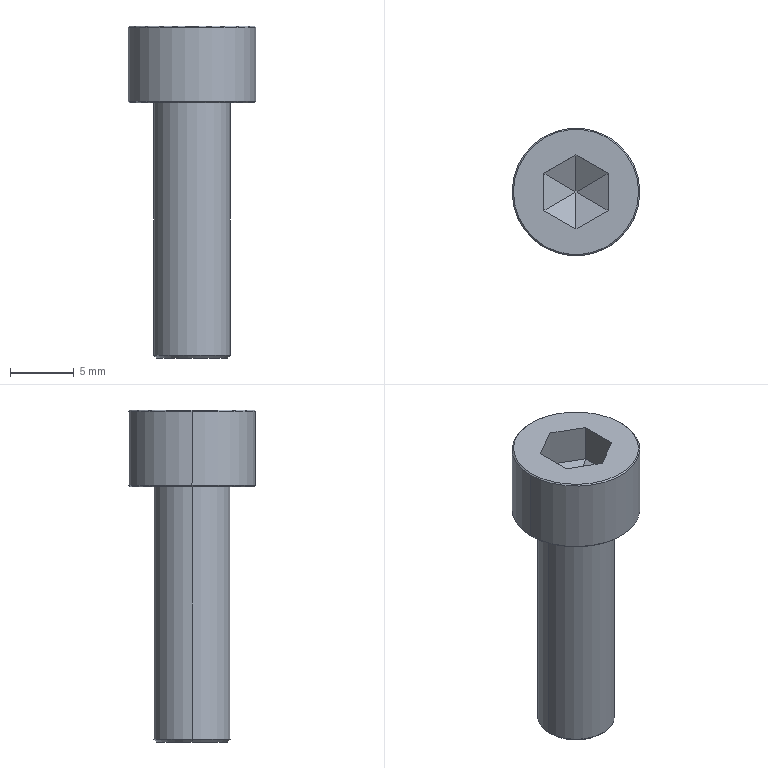Part | SolidWorks | features BaseBody 1 | 1 solid | 26 faces | box 10 x 10 x 26 mm | volume 959.271 mm3 | plane 16 | cone 6 | cylinder 4 | commonest cylinder face diameters 6 x2 10 x2
STEP:
#1=CARTESIAN_POINT('',(3.,0.,0.2));
#2=VERTEX_POINT('',#1);
#3=CARTESIAN_POINT('',(-3.,0.,0.2));
#4=VERTEX_POINT('',#3);
#5=CARTESIAN_POINT('',(0.,0.,0.2));
#6=DIRECTION('',(0.,0.,1.));
#7=DIRECTION('',(1.,0.,0.));
#8=AXIS2_PLACEMENT_3D('',#5,#6,#7);
#9=CIRCLE('',#8,3.);
#10=EDGE_CURVE('',#2,#4,#9,.T.);
#11=ORIENTED_EDGE('',*,*,#10,.T.);
#12=CARTESIAN_POINT('',(-3.,0.,20.));
#13=VERTEX_POINT('',#12);
#14=CARTESIAN_POINT('',(-3.,0.,0.));
#15=DIRECTION('',(0.,0.,1.));
#16=VECTOR('',#15,1000.);
#17=LINE('',#14,#16);
#18=EDGE_CURVE('',#4,#13,#17,.T.);
#19=ORIENTED_EDGE('',*,*,#18,.T.);
#20=CARTESIAN_POINT('',(3.,0.,20.));
#21=VERTEX_POINT('',#20);
#22=CARTESIAN_POINT('',(0.,0.,20.));
#23=DIRECTION('',(0.,0.,-1.));
#24=DIRECTION('',(1.,0.,0.));
#25=AXIS2_PLACEMENT_3D('',#22,#23,#24);
#26=CIRCLE('',#25,3.);
#27=EDGE_CURVE('',#13,#21,#26,.T.);
#28=ORIENTED_EDGE('',*,*,#27,.T.);
#29=CARTESIAN_POINT('',(3.,0.,0.));
#30=DIRECTION('',(0.,0.,1.));
#31=VECTOR('',#30,1000.);
#32=LINE('',#29,#31);
#33=EDGE_CURVE('',#2,#21,#32,.T.);
#34=ORIENTED_EDGE('',*,*,#33,.F.);
#35=EDGE_LOOP('',(#11,#19,#28,#34));
#36=FACE_OUTER_BOUND('',#35,.T.);
#37=CARTESIAN_POINT('',(0.,0.,0.));
#38=DIRECTION('',(0.,0.,1.));
#39=DIRECTION('',(1.,0.,0.));
#40=AXIS2_PLACEMENT_3D('',#37,#38,#39);
#41=CYLINDRICAL_SURFACE('',#40,3.);
#42=ADVANCED_FACE('',(#36),#41,.T.);
#43=CARTESIAN_POINT('',(2.8,0.,0.));
#44=VERTEX_POINT('',#43);
#45=CARTESIAN_POINT('',(-2.8,0.,0.));
#46=VERTEX_POINT('',#45);
#47=CARTESIAN_POINT('',(0.,0.,0.));
#48=DIRECTION('',(0.,0.,1.));
#49=DIRECTION('',(1.,0.,0.));
#50=AXIS2_PLACEMENT_3D('',#47,#48,#49);
#51=CIRCLE('',#50,2.8);
#52=EDGE_CURVE('',#44,#46,#51,.T.);
#53=ORIENTED_EDGE('',*,*,#52,.T.);
#54=CARTESIAN_POINT('',(-3.,0.,0.2));
#55=DIRECTION('',(-0.7071,0.,0.7071));
#56=VECTOR('',#55,1000.);
#57=LINE('',#54,#56);
#58=EDGE_CURVE('',#46,#4,#57,.T.);
#59=ORIENTED_EDGE('',*,*,#58,.T.);
#60=ORIENTED_EDGE('',*,*,#10,.F.);
#61=CARTESIAN_POINT('',(3.,0.,0.2));
#62=DIRECTION('',(0.7071,0.,0.7071));
#63=VECTOR('',#62,1000.);
#64=LINE('',#61,#63);
#65=EDGE_CURVE('',#44,#2,#64,.T.);
#66=ORIENTED_EDGE('',*,*,#65,.F.);
#67=EDGE_LOOP('',(#53,#59,#60,#66));
#68=FACE_OUTER_BOUND('',#67,.T.);
#69=CARTESIAN_POINT('',(0.,0.,0.2));
#70=DIRECTION('',(0.,0.,1.));
#71=DIRECTION('',(1.,0.,0.));
#72=AXIS2_PLACEMENT_3D('',#69,#70,#71);
#73=CONICAL_SURFACE('',#72,3.,0.7854);
#74=ADVANCED_FACE('',(#68),#73,.T.);
#75=CARTESIAN_POINT('',(4.9,0.,20.));
#76=VERTEX_POINT('',#75);
#77=CARTESIAN_POINT('',(-4.9,0.,20.));
#78=VERTEX_POINT('',#77);
#79=CARTESIAN_POINT('',(0.,0.,20.));
#80=DIRECTION('',(0.,0.,1.));
#81=DIRECTION('',(1.,0.,0.));
#82=AXIS2_PLACEMENT_3D('',#79,#80,#81);
#83=CIRCLE('',#82,4.9);
#84=EDGE_CURVE('',#76,#78,#83,.T.);
#85=ORIENTED_EDGE('',*,*,#84,.T.);
#86=CARTESIAN_POINT('',(-5.,0.,20.1));
#87=VERTEX_POINT('',#86);
#88=CARTESIAN_POINT('',(-5.,0.,20.1));
#89=DIRECTION('',(-0.7071,0.,0.7071));
#90=VECTOR('',#89,1000.);
#91=LINE('',#88,#90);
#92=EDGE_CURVE('',#78,#87,#91,.T.);
#93=ORIENTED_EDGE('',*,*,#92,.T.);
#94=CARTESIAN_POINT('',(5.,0.,20.1));
#95=VERTEX_POINT('',#94);
#96=CARTESIAN_POINT('',(0.,0.,20.1));
#97=DIRECTION('',(0.,0.,-1.));
#98=DIRECTION('',(0.,-1.,0.));
#99=AXIS2_PLACEMENT_3D('',#96,#97,#98);
#100=CIRCLE('',#99,5.);
#101=EDGE_CURVE('',#87,#95,#100,.T.);
#102=ORIENTED_EDGE('',*,*,#101,.T.);
#103=CARTESIAN_POINT('',(5.,0.,20.1));
#104=DIRECTION('',(0.7071,0.,0.7071));
#105=VECTOR('',#104,1000.);
#106=LINE('',#103,#105);
#107=EDGE_CURVE('',#76,#95,#106,.T.);
#108=ORIENTED_EDGE('',*,*,#107,.F.);
#109=EDGE_LOOP('',(#85,#93,#102,#108));
#110=FACE_OUTER_BOUND('',#109,.T.);
#111=CARTESIAN_POINT('',(0.,0.,20.1));
#112=DIRECTION('',(0.,0.,1.));
#113=DIRECTION('',(1.,0.,0.));
#114=AXIS2_PLACEMENT_3D('',#111,#112,#113);
#115=CONICAL_SURFACE('',#114,5.,0.7854);
#116=ADVANCED_FACE('',(#110),#115,.T.);
#117=ORIENTED_EDGE('',*,*,#101,.F.);
#118=CARTESIAN_POINT('',(-5.,0.,25.9));
#119=VERTEX_POINT('',#118);
#120=CARTESIAN_POINT('',(-5.,0.,20.));
#121=DIRECTION('',(0.,0.,1.));
#122=VECTOR('',#121,1000.);
#123=LINE('',#120,#122);
#124=EDGE_CURVE('',#87,#119,#123,.T.);
#125=ORIENTED_EDGE('',*,*,#124,.T.);
#126=CARTESIAN_POINT('',(5.,0.,25.9));
#127=VERTEX_POINT('',#126);
#128=CARTESIAN_POINT('',(0.,0.,25.9));
#129=DIRECTION('',(0.,0.,-1.));
#130=DIRECTION('',(1.,0.,0.));
#131=AXIS2_PLACEMENT_3D('',#128,#129,#130);
#132=CIRCLE('',#131,5.);
#133=EDGE_CURVE('',#119,#127,#132,.T.);
#134=ORIENTED_EDGE('',*,*,#133,.T.);
#135=CARTESIAN_POINT('',(5.,0.,20.));
#136=DIRECTION('',(0.,0.,1.));
#137=VECTOR('',#136,1000.);
#138=LINE('',#135,#137);
#139=EDGE_CURVE('',#95,#127,#138,.T.);
#140=ORIENTED_EDGE('',*,*,#139,.F.);
#141=EDGE_LOOP('',(#117,#125,#134,#140));
#142=FACE_OUTER_BOUND('',#141,.T.);
#143=CARTESIAN_POINT('',(0.,0.,20.));
#144=DIRECTION('',(0.,0.,1.));
#145=DIRECTION('',(1.,0.,0.));
#146=AXIS2_PLACEMENT_3D('',#143,#144,#145);
#147=CYLINDRICAL_SURFACE('',#146,5.);
#148=ADVANCED_FACE('',(#142),#147,.T.);
#149=CARTESIAN_POINT('',(-4.9,0.,26.));
#150=VERTEX_POINT('',#149);
#151=CARTESIAN_POINT('',(4.9,0.,26.));
#152=VERTEX_POINT('',#151);
#153=CARTESIAN_POINT('',(0.,0.,26.));
#154=DIRECTION('',(0.,0.,-1.));
#155=DIRECTION('',(1.,0.,0.));
#156=AXIS2_PLACEMENT_3D('',#153,#154,#155);
#157=CIRCLE('',#156,4.9);
#158=EDGE_CURVE('',#150,#152,#157,.T.);
#159=ORIENTED_EDGE('',*,*,#158,.T.);
#160=CARTESIAN_POINT('',(5.,0.,25.9));
#161=DIRECTION('',(0.7071,0.,-0.7071));
#162=VECTOR('',#161,1000.);
#163=LINE('',#160,#162);
#164=EDGE_CURVE('',#152,#127,#163,.T.);
#165=ORIENTED_EDGE('',*,*,#164,.T.);
#166=ORIENTED_EDGE('',*,*,#133,.F.);
#167=CARTESIAN_POINT('',(-5.,0.,25.9));
#168=DIRECTION('',(-0.7071,0.,-0.7071));
#169=VECTOR('',#168,1000.);
#170=LINE('',#167,#169);
#171=EDGE_CURVE('',#150,#119,#170,.T.);
#172=ORIENTED_EDGE('',*,*,#171,.F.);
#173=EDGE_LOOP('',(#159,#165,#166,#172));
#174=FACE_OUTER_BOUND('',#173,.T.);
#175=CARTESIAN_POINT('',(0.,0.,25.9));
#176=DIRECTION('',(0.,0.,-1.));
#177=DIRECTION('',(-1.,0.,0.));
#178=AXIS2_PLACEMENT_3D('',#175,#176,#177);
#179=CONICAL_SURFACE('',#178,5.,0.7854);
#180=ADVANCED_FACE('',(#174),#179,.T.);
#181=ORIENTED_EDGE('',*,*,#18,.F.);
#182=CARTESIAN_POINT('',(0.,0.,0.2));
#183=DIRECTION('',(0.,0.,1.));
#184=DIRECTION('',(1.,0.,0.));
#185=AXIS2_PLACEMENT_3D('',#182,#183,#184);
#186=CIRCLE('',#185,3.);
#187=EDGE_CURVE('',#4,#2,#186,.T.);
#188=ORIENTED_EDGE('',*,*,#187,.T.);
#189=ORIENTED_EDGE('',*,*,#33,.T.);
#190=CARTESIAN_POINT('',(0.,0.,20.));
#191=DIRECTION('',(0.,0.,-1.));
#192=DIRECTION('',(1.,0.,0.));
#193=AXIS2_PLACEMENT_3D('',#190,#191,#192);
#194=CIRCLE('',#193,3.);
#195=EDGE_CURVE('',#21,#13,#194,.T.);
#196=ORIENTED_EDGE('',*,*,#195,.T.);
#197=EDGE_LOOP('',(#181,#188,#189,#196));
#198=FACE_OUTER_BOUND('',#197,.T.);
#199=CARTESIAN_POINT('',(0.,0.,0.));
#200=DIRECTION('',(0.,0.,1.));
#201=DIRECTION('',(1.,0.,0.));
#202=AXIS2_PLACEMENT_3D('',#199,#200,#201);
#203=CYLINDRICAL_SURFACE('',#202,3.);
#204=ADVANCED_FACE('',(#198),#203,.T.);
#205=ORIENTED_EDGE('',*,*,#58,.F.);
#206=CARTESIAN_POINT('',(0.,0.,0.));
#207=DIRECTION('',(0.,0.,1.));
#208=DIRECTION('',(1.,0.,0.));
#209=AXIS2_PLACEMENT_3D('',#206,#207,#208);
#210=CIRCLE('',#209,2.8);
#211=EDGE_CURVE('',#46,#44,#210,.T.);
#212=ORIENTED_EDGE('',*,*,#211,.T.);
#213=ORIENTED_EDGE('',*,*,#65,.T.);
#214=ORIENTED_EDGE('',*,*,#187,.F.);
#215=EDGE_LOOP('',(#205,#212,#213,#214));
#216=FACE_OUTER_BOUND('',#215,.T.);
#217=CARTESIAN_POINT('',(0.,0.,0.2));
#218=DIRECTION('',(0.,0.,1.));
#219=DIRECTION('',(1.,0.,0.));
#220=AXIS2_PLACEMENT_3D('',#217,#218,#219);
#221=CONICAL_SURFACE('',#220,3.,0.7854);
#222=ADVANCED_FACE('',(#216),#221,.T.);
#223=ORIENTED_EDGE('',*,*,#195,.F.);
#224=ORIENTED_EDGE('',*,*,#27,.F.);
#225=EDGE_LOOP('',(#223,#224));
#226=FACE_BOUND('',#225,.T.);
#227=ORIENTED_EDGE('',*,*,#84,.F.);
#228=CARTESIAN_POINT('',(0.,0.,20.));
#229=DIRECTION('',(0.,0.,1.));
#230=DIRECTION('',(1.,0.,0.));
#231=AXIS2_PLACEMENT_3D('',#228,#229,#230);
#232=CIRCLE('',#231,4.9);
#233=EDGE_CURVE('',#78,#76,#232,.T.);
#234=ORIENTED_EDGE('',*,*,#233,.F.);
#235=EDGE_LOOP('',(#227,#234));
#236=FACE_OUTER_BOUND('',#235,.T.);
#237=CARTESIAN_POINT('',(0.,0.,20.));
#238=DIRECTION('',(0.,0.,1.));
#239=DIRECTION('',(1.,0.,0.));
#240=AXIS2_PLACEMENT_3D('',#237,#238,#239);
#241=PLANE('',#240);
#242=ADVANCED_FACE('',(#226,#236),#241,.F.);
#243=ORIENTED_EDGE('',*,*,#52,.F.);
#244=ORIENTED_EDGE('',*,*,#211,.F.);
#245=EDGE_LOOP('',(#243,#244));
#246=FACE_OUTER_BOUND('',#245,.T.);
#247=CARTESIAN_POINT('',(0.,0.,0.));
#248=DIRECTION('',(0.,0.,1.));
#249=DIRECTION('',(1.,0.,0.));
#250=AXIS2_PLACEMENT_3D('',#247,#248,#249);
#251=PLANE('',#250);
#252=ADVANCED_FACE('',(#246),#251,.F.);
#253=ORIENTED_EDGE('',*,*,#92,.F.);
#254=ORIENTED_EDGE('',*,*,#233,.T.);
#255=ORIENTED_EDGE('',*,*,#107,.T.);
#256=CARTESIAN_POINT('',(0.,0.,20.1));
#257=DIRECTION('',(0.,0.,-1.));
#258=DIRECTION('',(0.,-1.,0.));
#259=AXIS2_PLACEMENT_3D('',#256,#257,#258);
#260=CIRCLE('',#259,5.);
#261=EDGE_CURVE('',#95,#87,#260,.T.);
#262=ORIENTED_EDGE('',*,*,#261,.T.);
#263=EDGE_LOOP('',(#253,#254,#255,#262));
#264=FACE_OUTER_BOUND('',#263,.T.);
#265=CARTESIAN_POINT('',(0.,0.,20.1));
#266=DIRECTION('',(0.,0.,1.));
#267=DIRECTION('',(1.,0.,0.));
#268=AXIS2_PLACEMENT_3D('',#265,#266,#267);
#269=CONICAL_SURFACE('',#268,5.,0.7854);
#270=ADVANCED_FACE('',(#264),#269,.T.);
#271=ORIENTED_EDGE('',*,*,#124,.F.);
#272=ORIENTED_EDGE('',*,*,#261,.F.);
#273=ORIENTED_EDGE('',*,*,#139,.T.);
#274=CARTESIAN_POINT('',(0.,0.,25.9));
#275=DIRECTION('',(0.,0.,-1.));
#276=DIRECTION('',(1.,0.,0.));
#277=AXIS2_PLACEMENT_3D('',#274,#275,#276);
#278=CIRCLE('',#277,5.);
#279=EDGE_CURVE('',#127,#119,#278,.T.);
#280=ORIENTED_EDGE('',*,*,#279,.T.);
#281=EDGE_LOOP('',(#271,#272,#273,#280));
#282=FACE_OUTER_BOUND('',#281,.T.);
#283=CARTESIAN_POINT('',(0.,0.,20.));
#284=DIRECTION('',(0.,0.,1.));
#285=DIRECTION('',(1.,0.,0.));
#286=AXIS2_PLACEMENT_3D('',#283,#284,#285);
#287=CYLINDRICAL_SURFACE('',#286,5.);
#288=ADVANCED_FACE('',(#282),#287,.T.);
#289=ORIENTED_EDGE('',*,*,#164,.F.);
#290=CARTESIAN_POINT('',(0.,0.,26.));
#291=DIRECTION('',(0.,0.,-1.));
#292=DIRECTION('',(1.,0.,0.));
#293=AXIS2_PLACEMENT_3D('',#290,#291,#292);
#294=CIRCLE('',#293,4.9);
#295=EDGE_CURVE('',#152,#150,#294,.T.);
#296=ORIENTED_EDGE('',*,*,#295,.T.);
#297=ORIENTED_EDGE('',*,*,#171,.T.);
#298=ORIENTED_EDGE('',*,*,#279,.F.);
#299=EDGE_LOOP('',(#289,#296,#297,#298));
#300=FACE_OUTER_BOUND('',#299,.T.);
#301=CARTESIAN_POINT('',(0.,0.,25.9));
#302=DIRECTION('',(0.,0.,-1.));
#303=DIRECTION('',(-1.,0.,0.));
#304=AXIS2_PLACEMENT_3D('',#301,#302,#303);
#305=CONICAL_SURFACE('',#304,5.,0.7854);
#306=ADVANCED_FACE('',(#300),#305,.T.);
#307=CARTESIAN_POINT('',(-2.51,-1.449,26.));
#308=VERTEX_POINT('',#307);
#309=CARTESIAN_POINT('',(-2.51,1.449,26.));
#310=VERTEX_POINT('',#309);
#311=CARTESIAN_POINT('',(-2.51,0.,26.));
#312=DIRECTION('',(0.,1.,0.));
#313=VECTOR('',#312,1000.);
#314=LINE('',#311,#313);
#315=EDGE_CURVE('',#308,#310,#314,.T.);
#316=ORIENTED_EDGE('',*,*,#315,.T.);
#317=CARTESIAN_POINT('',(0.,2.898,26.));
#318=VERTEX_POINT('',#317);
#319=CARTESIAN_POINT('',(-2.51,1.449,26.));
#320=DIRECTION('',(0.866,0.5,0.));
#321=VECTOR('',#320,1000.);
#322=LINE('',#319,#321);
#323=EDGE_CURVE('',#310,#318,#322,.T.);
#324=ORIENTED_EDGE('',*,*,#323,.T.);
#325=CARTESIAN_POINT('',(2.51,1.449,26.));
#326=VERTEX_POINT('',#325);
#327=CARTESIAN_POINT('',(0.,2.898,26.));
#328=DIRECTION('',(0.866,-0.5,0.));
#329=VECTOR('',#328,1000.);
#330=LINE('',#327,#329);
#331=EDGE_CURVE('',#318,#326,#330,.T.);
#332=ORIENTED_EDGE('',*,*,#331,.T.);
#333=CARTESIAN_POINT('',(2.51,-1.449,26.));
#334=VERTEX_POINT('',#333);
#335=CARTESIAN_POINT('',(2.51,0.,26.));
#336=DIRECTION('',(0.,-1.,0.));
#337=VECTOR('',#336,1000.);
#338=LINE('',#335,#337);
#339=EDGE_CURVE('',#326,#334,#338,.T.);
#340=ORIENTED_EDGE('',*,*,#339,.T.);
#341=CARTESIAN_POINT('',(0.,-2.898,26.));
#342=VERTEX_POINT('',#341);
#343=CARTESIAN_POINT('',(2.51,-1.449,26.));
#344=DIRECTION('',(-0.866,-0.5,0.));
#345=VECTOR('',#344,1000.);
#346=LINE('',#343,#345);
#347=EDGE_CURVE('',#334,#342,#346,.T.);
#348=ORIENTED_EDGE('',*,*,#347,.T.);
#349=CARTESIAN_POINT('',(0.,-2.898,26.));
#350=DIRECTION('',(-0.866,0.5,0.));
#351=VECTOR('',#350,1000.);
#352=LINE('',#349,#351);
#353=EDGE_CURVE('',#342,#308,#352,.T.);
#354=ORIENTED_EDGE('',*,*,#353,.T.);
#355=EDGE_LOOP('',(#316,#324,#332,#340,#348,#354));
#356=FACE_BOUND('',#355,.T.);
#357=ORIENTED_EDGE('',*,*,#158,.F.);
#358=ORIENTED_EDGE('',*,*,#295,.F.);
#359=EDGE_LOOP('',(#357,#358));
#360=FACE_OUTER_BOUND('',#359,.T.);
#361=CARTESIAN_POINT('',(0.,0.,26.));
#362=DIRECTION('',(0.,0.,1.));
#363=DIRECTION('',(1.,0.,0.));
#364=AXIS2_PLACEMENT_3D('',#361,#362,#363);
#365=PLANE('',#364);
#366=ADVANCED_FACE('',(#356,#360),#365,.T.);
#367=ORIENTED_EDGE('',*,*,#323,.F.);
#368=CARTESIAN_POINT('',(-2.51,1.449,23.));
#369=VERTEX_POINT('',#368);
#370=CARTESIAN_POINT('',(-2.51,1.449,26.));
#371=DIRECTION('',(0.,0.,1.));
#372=VECTOR('',#371,1000.);
#373=LINE('',#370,#372);
#374=EDGE_CURVE('',#369,#310,#373,.T.);
#375=ORIENTED_EDGE('',*,*,#374,.F.);
#376=CARTESIAN_POINT('',(0.,2.898,23.));
#377=VERTEX_POINT('',#376);
#378=CARTESIAN_POINT('',(0.,2.898,23.));
#379=DIRECTION('',(-0.866,-0.5,0.));
#380=VECTOR('',#379,1000.);
#381=LINE('',#378,#380);
#382=EDGE_CURVE('',#377,#369,#381,.T.);
#383=ORIENTED_EDGE('',*,*,#382,.F.);
#384=CARTESIAN_POINT('',(0.,2.898,26.));
#385=DIRECTION('',(0.,0.,-1.));
#386=VECTOR('',#385,1000.);
#387=LINE('',#384,#386);
#388=EDGE_CURVE('',#318,#377,#387,.T.);
#389=ORIENTED_EDGE('',*,*,#388,.F.);
#390=EDGE_LOOP('',(#367,#375,#383,#389));
#391=FACE_OUTER_BOUND('',#390,.T.);
#392=CARTESIAN_POINT('',(0.,2.898,26.));
#393=DIRECTION('',(-0.5,0.866,0.));
#394=DIRECTION('',(-0.866,-0.5,0.));
#395=AXIS2_PLACEMENT_3D('',#392,#393,#394);
#396=PLANE('',#395);
#397=ADVANCED_FACE('',(#391),#396,.F.);
#398=ORIENTED_EDGE('',*,*,#315,.F.);
#399=CARTESIAN_POINT('',(-2.51,-1.449,23.));
#400=VERTEX_POINT('',#399);
#401=CARTESIAN_POINT('',(-2.51,-1.449,26.));
#402=DIRECTION('',(0.,0.,1.));
#403=VECTOR('',#402,1000.);
#404=LINE('',#401,#403);
#405=EDGE_CURVE('',#400,#308,#404,.T.);
#406=ORIENTED_EDGE('',*,*,#405,.F.);
#407=CARTESIAN_POINT('',(-2.51,1.449,23.));
#408=DIRECTION('',(0.,-1.,0.));
#409=VECTOR('',#408,1000.);
#410=LINE('',#407,#409);
#411=EDGE_CURVE('',#369,#400,#410,.T.);
#412=ORIENTED_EDGE('',*,*,#411,.F.);
#413=ORIENTED_EDGE('',*,*,#374,.T.);
#414=EDGE_LOOP('',(#398,#406,#412,#413));
#415=FACE_OUTER_BOUND('',#414,.T.);
#416=CARTESIAN_POINT('',(-2.51,1.449,26.));
#417=DIRECTION('',(-1.,0.,0.));
#418=DIRECTION('',(0.,0.,1.));
#419=AXIS2_PLACEMENT_3D('',#416,#417,#418);
#420=PLANE('',#419);
#421=ADVANCED_FACE('',(#415),#420,.F.);
#422=ORIENTED_EDGE('',*,*,#353,.F.);
#423=CARTESIAN_POINT('',(0.,-2.898,23.));
#424=VERTEX_POINT('',#423);
#425=CARTESIAN_POINT('',(0.,-2.898,26.));
#426=DIRECTION('',(0.,0.,1.));
#427=VECTOR('',#426,1000.);
#428=LINE('',#425,#427);
#429=EDGE_CURVE('',#424,#342,#428,.T.);
#430=ORIENTED_EDGE('',*,*,#429,.F.);
#431=CARTESIAN_POINT('',(-2.51,-1.449,23.));
#432=DIRECTION('',(0.866,-0.5,0.));
#433=VECTOR('',#432,1000.);
#434=LINE('',#431,#433);
#435=EDGE_CURVE('',#400,#424,#434,.T.);
#436=ORIENTED_EDGE('',*,*,#435,.F.);
#437=ORIENTED_EDGE('',*,*,#405,.T.);
#438=EDGE_LOOP('',(#422,#430,#436,#437));
#439=FACE_OUTER_BOUND('',#438,.T.);
#440=CARTESIAN_POINT('',(-2.51,-1.449,26.));
#441=DIRECTION('',(-0.5,-0.866,0.));
#442=DIRECTION('',(0.866,-0.5,0.));
#443=AXIS2_PLACEMENT_3D('',#440,#441,#442);
#444=PLANE('',#443);
#445=ADVANCED_FACE('',(#439),#444,.F.);
#446=ORIENTED_EDGE('',*,*,#347,.F.);
#447=CARTESIAN_POINT('',(2.51,-1.449,23.));
#448=VERTEX_POINT('',#447);
#449=CARTESIAN_POINT('',(2.51,-1.449,26.));
#450=DIRECTION('',(0.,0.,1.));
#451=VECTOR('',#450,1000.);
#452=LINE('',#449,#451);
#453=EDGE_CURVE('',#448,#334,#452,.T.);
#454=ORIENTED_EDGE('',*,*,#453,.F.);
#455=CARTESIAN_POINT('',(0.,-2.898,23.));
#456=DIRECTION('',(0.866,0.5,0.));
#457=VECTOR('',#456,1000.);
#458=LINE('',#455,#457);
#459=EDGE_CURVE('',#424,#448,#458,.T.);
#460=ORIENTED_EDGE('',*,*,#459,.F.);
#461=ORIENTED_EDGE('',*,*,#429,.T.);
#462=EDGE_LOOP('',(#446,#454,#460,#461));
#463=FACE_OUTER_BOUND('',#462,.T.);
#464=CARTESIAN_POINT('',(0.,-2.898,26.));
#465=DIRECTION('',(0.5,-0.866,0.));
#466=DIRECTION('',(0.866,0.5,0.));
#467=AXIS2_PLACEMENT_3D('',#464,#465,#466);
#468=PLANE('',#467);
#469=ADVANCED_FACE('',(#463),#468,.F.);
#470=ORIENTED_EDGE('',*,*,#339,.F.);
#471=CARTESIAN_POINT('',(2.51,1.449,23.));
#472=VERTEX_POINT('',#471);
#473=CARTESIAN_POINT('',(2.51,1.449,26.));
#474=DIRECTION('',(0.,0.,1.));
#475=VECTOR('',#474,1000.);
#476=LINE('',#473,#475);
#477=EDGE_CURVE('',#472,#326,#476,.T.);
#478=ORIENTED_EDGE('',*,*,#477,.F.);
#479=CARTESIAN_POINT('',(2.51,-1.449,23.));
#480=DIRECTION('',(0.,1.,0.));
#481=VECTOR('',#480,1000.);
#482=LINE('',#479,#481);
#483=EDGE_CURVE('',#448,#472,#482,.T.);
#484=ORIENTED_EDGE('',*,*,#483,.F.);
#485=ORIENTED_EDGE('',*,*,#453,.T.);
#486=EDGE_LOOP('',(#470,#478,#484,#485));
#487=FACE_OUTER_BOUND('',#486,.T.);
#488=CARTESIAN_POINT('',(2.51,-1.449,26.));
#489=DIRECTION('',(1.,0.,0.));
#490=DIRECTION('',(0.,0.,-1.));
#491=AXIS2_PLACEMENT_3D('',#488,#489,#490);
#492=PLANE('',#491);
#493=ADVANCED_FACE('',(#487),#492,.F.);
#494=ORIENTED_EDGE('',*,*,#331,.F.);
#495=ORIENTED_EDGE('',*,*,#388,.T.);
#496=CARTESIAN_POINT('',(2.51,1.449,23.));
#497=DIRECTION('',(-0.866,0.5,0.));
#498=VECTOR('',#497,1000.);
#499=LINE('',#496,#498);
#500=EDGE_CURVE('',#472,#377,#499,.T.);
#501=ORIENTED_EDGE('',*,*,#500,.F.);
#502=ORIENTED_EDGE('',*,*,#477,.T.);
#503=EDGE_LOOP('',(#494,#495,#501,#502));
#504=FACE_OUTER_BOUND('',#503,.T.);
#505=CARTESIAN_POINT('',(2.51,1.449,26.));
#506=DIRECTION('',(0.5,0.866,0.));
#507=DIRECTION('',(-0.866,0.5,0.));
#508=AXIS2_PLACEMENT_3D('',#505,#506,#507);
#509=PLANE('',#508);
#510=ADVANCED_FACE('',(#504),#509,.F.);
#511=CARTESIAN_POINT('',(0.,0.1,21.5));
#512=VERTEX_POINT('',#511);
#513=CARTESIAN_POINT('',(-0.0866,0.05,21.5));
#514=VERTEX_POINT('',#513);
#515=CARTESIAN_POINT('',(0.,0.1,21.5));
#516=DIRECTION('',(-0.866,-0.5,0.));
#517=VECTOR('',#516,1000.);
#518=LINE('',#515,#517);
#519=EDGE_CURVE('',#512,#514,#518,.T.);
#520=ORIENTED_EDGE('',*,*,#519,.F.);
#521=CARTESIAN_POINT('',(0.,1.208,22.094));
#522=DIRECTION('',(0.,-0.8814,-0.4724));
#523=VECTOR('',#522,1000.);
#524=LINE('',#521,#523);
#525=EDGE_CURVE('',#377,#512,#524,.T.);
#526=ORIENTED_EDGE('',*,*,#525,.F.);
#527=ORIENTED_EDGE('',*,*,#382,.T.);
#528=CARTESIAN_POINT('',(-0.0866,0.05,21.5));
#529=DIRECTION('',(-0.7633,0.4407,0.4724));
#530=VECTOR('',#529,1000.);
#531=LINE('',#528,#530);
#532=EDGE_CURVE('',#514,#369,#531,.T.);
#533=ORIENTED_EDGE('',*,*,#532,.F.);
#534=EDGE_LOOP('',(#520,#526,#527,#533));
#535=FACE_OUTER_BOUND('',#534,.T.);
#536=CARTESIAN_POINT('',(-0.6492,1.124,22.25));
#537=DIRECTION('',(-0.2632,0.4558,-0.8503));
#538=DIRECTION('',(0.,0.8814,0.4724));
#539=AXIS2_PLACEMENT_3D('',#536,#537,#538);
#540=PLANE('',#539);
#541=ADVANCED_FACE('',(#535),#540,.F.);
#542=CARTESIAN_POINT('',(-0.0866,-0.05,21.5));
#543=VERTEX_POINT('',#542);
#544=CARTESIAN_POINT('',(-0.0866,0.,21.5));
#545=DIRECTION('',(0.,-1.,0.));
#546=VECTOR('',#545,1000.);
#547=LINE('',#544,#546);
#548=EDGE_CURVE('',#514,#543,#547,.T.);
#549=ORIENTED_EDGE('',*,*,#548,.F.);
#550=ORIENTED_EDGE('',*,*,#532,.T.);
#551=ORIENTED_EDGE('',*,*,#411,.T.);
#552=CARTESIAN_POINT('',(-0.0866,-0.05,21.5));
#553=DIRECTION('',(-0.7633,-0.4407,0.4724));
#554=VECTOR('',#553,1000.);
#555=LINE('',#552,#554);
#556=EDGE_CURVE('',#543,#400,#555,.T.);
#557=ORIENTED_EDGE('',*,*,#556,.F.);
#558=EDGE_LOOP('',(#549,#550,#551,#557));
#559=FACE_OUTER_BOUND('',#558,.T.);
#560=CARTESIAN_POINT('',(-1.298,0.,22.25));
#561=DIRECTION('',(-0.5263,0.,-0.8503));
#562=DIRECTION('',(-0.8503,0.,0.5263));
#563=AXIS2_PLACEMENT_3D('',#560,#561,#562);
#564=PLANE('',#563);
#565=ADVANCED_FACE('',(#559),#564,.F.);
#566=CARTESIAN_POINT('',(0.,-0.1,21.5));
#567=VERTEX_POINT('',#566);
#568=CARTESIAN_POINT('',(-0.0866,-0.05,21.5));
#569=DIRECTION('',(0.866,-0.5,0.));
#570=VECTOR('',#569,1000.);
#571=LINE('',#568,#570);
#572=EDGE_CURVE('',#543,#567,#571,.T.);
#573=ORIENTED_EDGE('',*,*,#572,.F.);
#574=ORIENTED_EDGE('',*,*,#556,.T.);
#575=ORIENTED_EDGE('',*,*,#435,.T.);
#576=CARTESIAN_POINT('',(0.,-1.208,22.094));
#577=DIRECTION('',(0.,-0.8814,0.4724));
#578=VECTOR('',#577,1000.);
#579=LINE('',#576,#578);
#580=EDGE_CURVE('',#567,#424,#579,.T.);
#581=ORIENTED_EDGE('',*,*,#580,.F.);
#582=EDGE_LOOP('',(#573,#574,#575,#581));
#583=FACE_OUTER_BOUND('',#582,.T.);
#584=CARTESIAN_POINT('',(-0.6492,-1.124,22.25));
#585=DIRECTION('',(-0.2632,-0.4558,-0.8503));
#586=DIRECTION('',(0.,0.8814,-0.4724));
#587=AXIS2_PLACEMENT_3D('',#584,#585,#586);
#588=PLANE('',#587);
#589=ADVANCED_FACE('',(#583),#588,.F.);
#590=CARTESIAN_POINT('',(0.0866,-0.05,21.5));
#591=VERTEX_POINT('',#590);
#592=CARTESIAN_POINT('',(0.,-0.1,21.5));
#593=DIRECTION('',(0.866,0.5,0.));
#594=VECTOR('',#593,1000.);
#595=LINE('',#592,#594);
#596=EDGE_CURVE('',#567,#591,#595,.T.);
#597=ORIENTED_EDGE('',*,*,#596,.F.);
#598=ORIENTED_EDGE('',*,*,#580,.T.);
#599=ORIENTED_EDGE('',*,*,#459,.T.);
#600=CARTESIAN_POINT('',(0.0866,-0.05,21.5));
#601=DIRECTION('',(0.7633,-0.4407,0.4724));
#602=VECTOR('',#601,1000.);
#603=LINE('',#600,#602);
#604=EDGE_CURVE('',#591,#448,#603,.T.);
#605=ORIENTED_EDGE('',*,*,#604,.F.);
#606=EDGE_LOOP('',(#597,#598,#599,#605));
#607=FACE_OUTER_BOUND('',#606,.T.);
#608=CARTESIAN_POINT('',(0.6492,-1.124,22.25));
#609=DIRECTION('',(0.2632,-0.4558,-0.8503));
#610=DIRECTION('',(0.,0.8814,-0.4724));
#611=AXIS2_PLACEMENT_3D('',#608,#609,#610);
#612=PLANE('',#611);
#613=ADVANCED_FACE('',(#607),#612,.F.);
#614=CARTESIAN_POINT('',(0.0866,0.05,21.5));
#615=VERTEX_POINT('',#614);
#616=CARTESIAN_POINT('',(0.0866,0.,21.5));
#617=DIRECTION('',(0.,1.,0.));
#618=VECTOR('',#617,1000.);
#619=LINE('',#616,#618);
#620=EDGE_CURVE('',#591,#615,#619,.T.);
#621=ORIENTED_EDGE('',*,*,#620,.F.);
#622=ORIENTED_EDGE('',*,*,#604,.T.);
#623=ORIENTED_EDGE('',*,*,#483,.T.);
#624=CARTESIAN_POINT('',(0.0866,0.05,21.5));
#625=DIRECTION('',(0.7633,0.4407,0.4724));
#626=VECTOR('',#625,1000.);
#627=LINE('',#624,#626);
#628=EDGE_CURVE('',#615,#472,#627,.T.);
#629=ORIENTED_EDGE('',*,*,#628,.F.);
#630=EDGE_LOOP('',(#621,#622,#623,#629));
#631=FACE_OUTER_BOUND('',#630,.T.);
#632=CARTESIAN_POINT('',(1.298,0.,22.25));
#633=DIRECTION('',(0.5263,0.,-0.8503));
#634=DIRECTION('',(-0.8503,0.,-0.5263));
#635=AXIS2_PLACEMENT_3D('',#632,#633,#634);
#636=PLANE('',#635);
#637=ADVANCED_FACE('',(#631),#636,.F.);
#638=CARTESIAN_POINT('',(0.0866,0.05,21.5));
#639=DIRECTION('',(-0.866,0.5,0.));
#640=VECTOR('',#639,1000.);
#641=LINE('',#638,#640);
#642=EDGE_CURVE('',#615,#512,#641,.T.);
#643=ORIENTED_EDGE('',*,*,#642,.F.);
#644=ORIENTED_EDGE('',*,*,#628,.T.);
#645=ORIENTED_EDGE('',*,*,#500,.T.);
#646=ORIENTED_EDGE('',*,*,#525,.T.);
#647=EDGE_LOOP('',(#643,#644,#645,#646));
#648=FACE_OUTER_BOUND('',#647,.T.);
#649=CARTESIAN_POINT('',(0.6492,1.124,22.25));
#650=DIRECTION('',(0.2632,0.4558,-0.8503));
#651=DIRECTION('',(0.,0.8814,0.4724));
#652=AXIS2_PLACEMENT_3D('',#649,#650,#651);
#653=PLANE('',#652);
#654=ADVANCED_FACE('',(#648),#653,.F.);
#655=ORIENTED_EDGE('',*,*,#596,.T.);
#656=ORIENTED_EDGE('',*,*,#620,.T.);
#657=ORIENTED_EDGE('',*,*,#642,.T.);
#658=ORIENTED_EDGE('',*,*,#519,.T.);
#659=ORIENTED_EDGE('',*,*,#548,.T.);
#660=ORIENTED_EDGE('',*,*,#572,.T.);
#661=EDGE_LOOP('',(#655,#656,#657,#658,#659,#660));
#662=FACE_OUTER_BOUND('',#661,.T.);
#663=CARTESIAN_POINT('',(0.,0.,21.5));
#664=DIRECTION('',(0.,0.,1.));
#665=DIRECTION('',(1.,0.,0.));
#666=AXIS2_PLACEMENT_3D('',#663,#664,#665);
#667=PLANE('',#666);
#668=ADVANCED_FACE('',(#662),#667,.T.);
#669=CLOSED_SHELL('',(#42,#74,#116,#148,#180,#204,#222,#242,#252,#270,#288,#306,#366,#397,#421,#445,#469,#493,#510,#541,#565,#589,#613,#637,#654,#668));
#670=MANIFOLD_SOLID_BREP('',#669);
#671=CARTESIAN_POINT('',(0.,0.,0.));
#672=DIRECTION('',(0.,0.,1.));
#673=DIRECTION('',(1.,0.,0.));
#674=AXIS2_PLACEMENT_3D('',#671,#672,#673);
#675=(LENGTH_UNIT()NAMED_UNIT(*)SI_UNIT(.MILLI.,.METRE.));
#676=UNCERTAINTY_MEASURE_WITH_UNIT(LENGTH_MEASURE(0.00001),#675,'','');
#677=(NAMED_UNIT(*)PLANE_ANGLE_UNIT()SI_UNIT($,.RADIAN.));
#678=(NAMED_UNIT(*)SI_UNIT($,.STERADIAN.)SOLID_ANGLE_UNIT());
#679=(GEOMETRIC_REPRESENTATION_CONTEXT(3)GLOBAL_UNCERTAINTY_ASSIGNED_CONTEXT((#676))GLOBAL_UNIT_ASSIGNED_CONTEXT((#675,#677,#678))REPRESENTATION_CONTEXT('',''));
#680=ADVANCED_BREP_SHAPE_REPRESENTATION('',(#670,#674),#679);